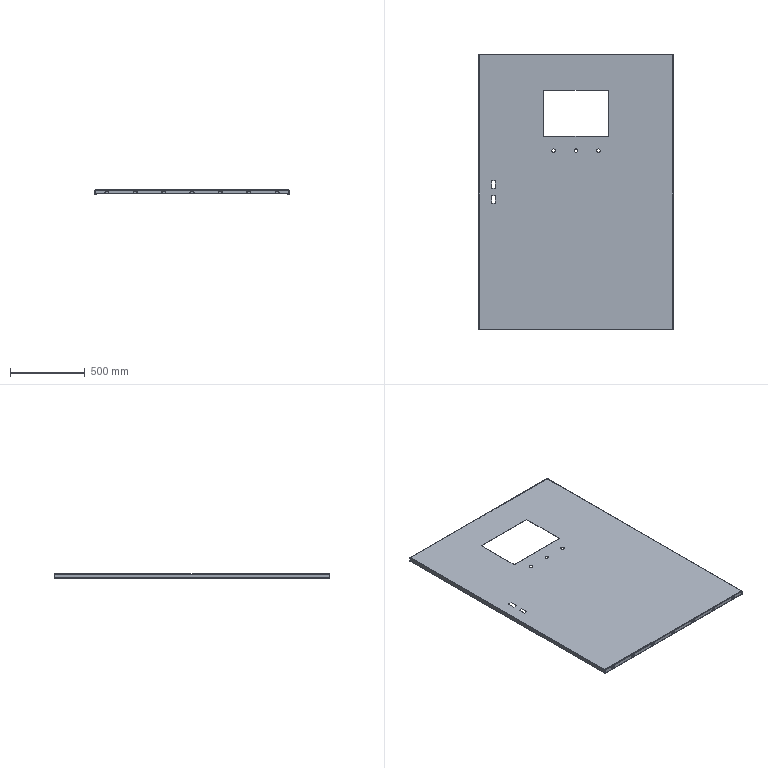Part | SolidWorks | features BaseBody 1 | 1 solid | 236 faces | box 1300 x 1846 x 30 mm | volume 5026175 mm3 | plane 173 | cylinder 63 | commonest cylinder face diameters 10 x14 12 x14 2 x11 6 x11 22.5 x9 0.1 x2